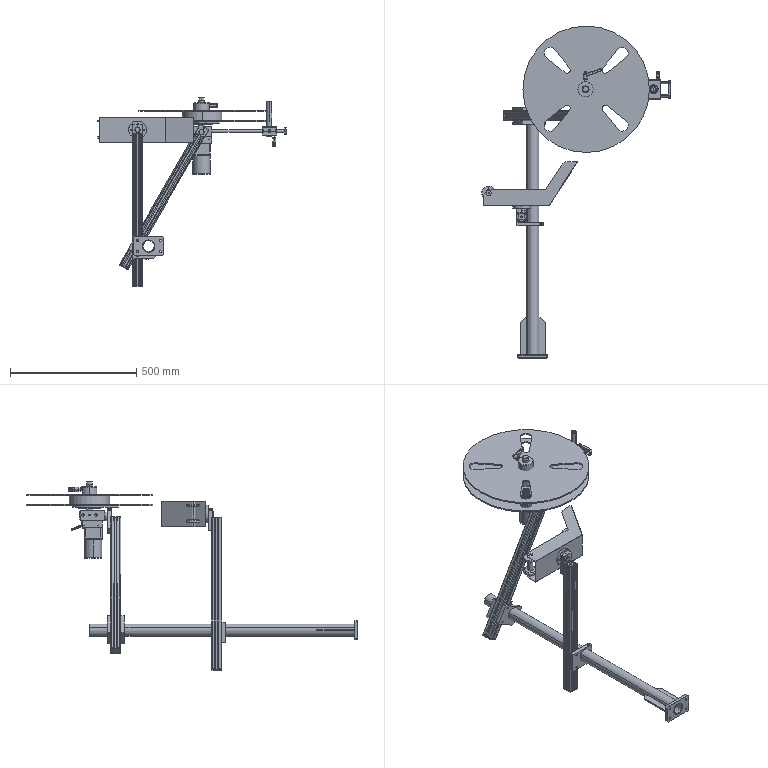Part | NX | 43 solids | 1494 faces | box 745.641 x 1312 x 743.277 mm | volume 6126186 mm3 | cylinder 582 | plane 522 | cone 293 | torus 57 | spline 30 | sphere 10 | commonest cylinder face diameters 4.2 x44 10 x39 8 x36 6.5 x28 25 x28 19 x26